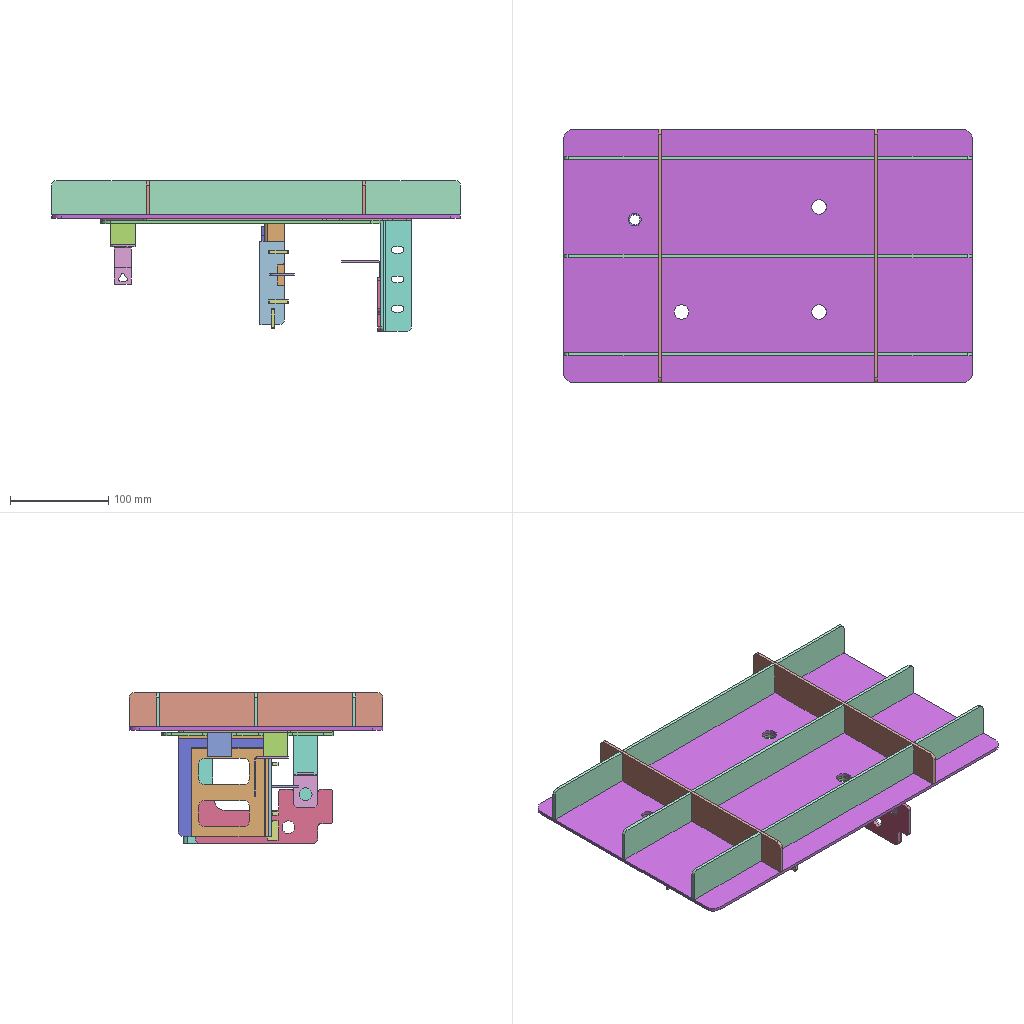Assembly | SolidWorks | 15 different items | 21 placed | box 416 x 258 x 153 mm
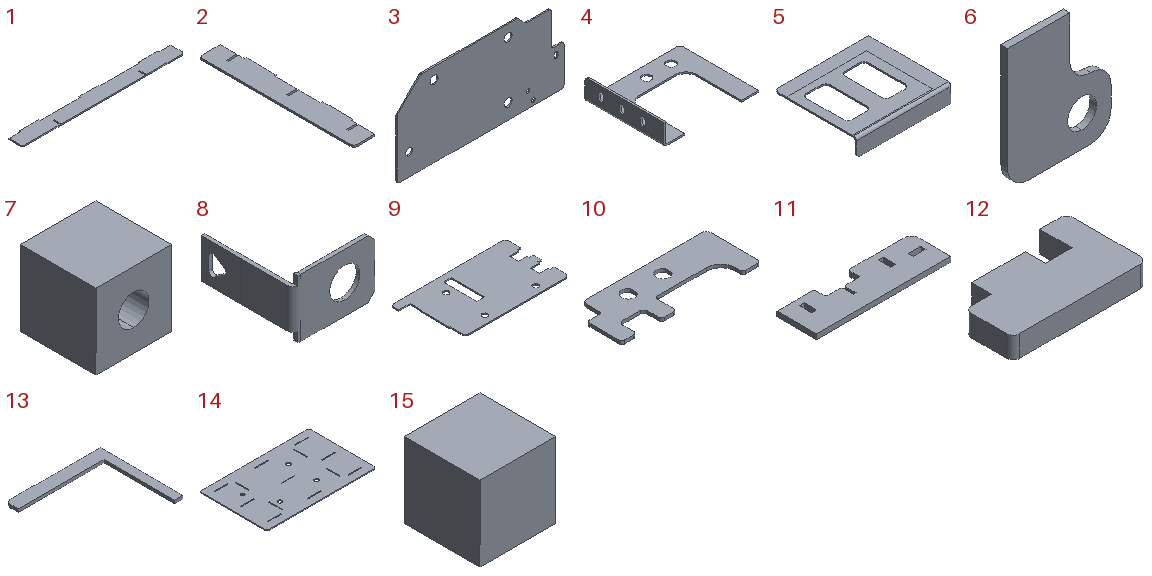Parts list (item | quantity | size | volume | features):
1 | x3 | 416 x 38 x 3.2 mm | 47629 mm3 | features FlatPattern 1, SMBaseFlange 1, SheetMetal 1
2 | x2 | 38 x 258 x 3.2 mm | 29284 mm3 | features FlatPattern 1, SMBaseFlange 1, SheetMetal 1
3 | x1 | 316 x 2.3 x 158 mm | 104007 mm3 | features FlatPattern 1, SMBaseFlange 1, SheetMetal 1
4 | x1 | 137 x 113 x 31 mm | 26668 mm3 | features ICE 2, Fillet 1, FlatPattern 1, SMBaseFlange 1, SheetMetal 1
5 | x1 | 106 x 92 x 20 mm | 14216 mm3 | features ICE 3, Fillet 1, FlatPattern 1, SMBaseFlange 1, SheetMetal 1
6 | x1 | 25 x 1.6 x 30 mm | 881.257 mm3 | features Fillet 1, FlatPattern 1, SMBaseFlange 1, SheetMetal 1
7 | x1 | 25 x 25 x 25 mm | 13582 mm3 | features Extrusion 1, HoleWzd 1
8 | x2 | 35 x 40 x 25 mm | 2088 mm3 | features ICE 5, Chamfer 1, FlatPattern 1, SMBaseFlange 1, SheetMetal 1
9 | x1 | 316 x 175 x 3.2 mm | 147992 mm3 | features FlatPattern 1, SMBaseFlange 1, SheetMetal 1
10 | x1 | 140 x 55 x 3.2 mm | 16813 mm3 | features FlatPattern 1, SMBaseFlange 1, SheetMetal 1
11 | x1 | 85 x 25 x 3.2 mm | 5979 mm3 | features FlatPattern 1, SMBaseFlange 1, SheetMetal 1
12 | x3 | 20 x 12 x 3.2 mm | 596.293 mm3 | features FlatPattern 1, SMBaseFlange 1, SheetMetal 1
13 | x1 | 100 x 88 x 3.2 mm | 6303 mm3 | features FlatPattern 1, SMBaseFlange 1, SheetMetal 1
14 | x1 | 416 x 258 x 3.2 mm | 334398 mm3 | features FlatPattern 1, SMBaseFlange 1, SheetMetal 1
15 | x1 | 25 x 25 x 25 mm | 15625 mm3 | features Extrusion 1
Mates (type | each side: item.copy, entity, surface, feature):
Coincident | 3.1 face plane Base-Flange1 | 7.1 face plane Boss-Extrude1
Concentric | 3.1 face cylinder Base-Flange1 | 7.1 face cylinder M12 Tapped Hole1
Parallel | 3.1 face plane Base-Flange1 | 7.1 face plane Boss-Extrude1
Coincident | 3.1 face plane Base-Flange1 | 15.1 face plane Boss-Extrude1
Coincident | 7.1 face plane Boss-Extrude1 | 15.1 face plane Boss-Extrude1
DistanceDim | 7.1 face plane Boss-Extrude1 | 15.1 face plane Boss-Extrude1
Coincident | 15.1 face plane Boss-Extrude1 | 8.1 face plane Base-Flange1 | 2 times
DistanceDim | 8.1 face cylinder Cut-Extrude3 | 15.1 face plane Boss-Extrude1
Coincident | 3.1 face plane Base-Flange1 | 4.1 face plane Base-Flange1 | 2 times
DistanceDim | 4.1 face plane Base-Flange1 | 3.1 face plane Base-Flange1
Coincident | 4.1 face plane Base-Flange1 | 8.2 face plane Base-Flange1 | 2 times
DistanceDim | 8.2 face cylinder Cut-Extrude3 | 4.1 face plane Base-Flange1
Coincident | 3.1 face plane Base-Flange1 | 5.1 face plane Base-Flange1 | 2 times
DistanceDim | 5.1 face plane Base-Flange1 | 3.1 face plane Base-Flange1
Coincident | 5.1 face plane Base-Flange1 | 6.1 face plane Base-Flange1
DistanceDim | 5.1 face plane Base-Flange1 | 6.1 face plane Base-Flange1
DistanceDim | 6.1 face plane Base-Flange1 | 5.1 face plane Base-Flange1
InPlace | 3.1 face plane Base-Flange1 | 9.1 plane
InPlace | 4.1 face plane Base-Flange1 | 10.1 plane
InPlace | 5.1 face plane Base-Flange1 | 11.1 plane
InPlace | 12.1 plane | assembly plane
Coincident | 11.1 face plane Base-Flange1 | 12.2 face plane Base-Flange1 | 2 times
DistanceDim | 11.1 face plane Base-Flange1 | 12.2 face plane Base-Flange1
InPlace | 3.1 face plane Base-Flange1 | 14.1 plane
InPlace | 1.1 plane | assembly plane
InPlace | 2.1 plane | assembly plane
InPlace | 5.1 face plane Base-Flange1 | 13.1 plane